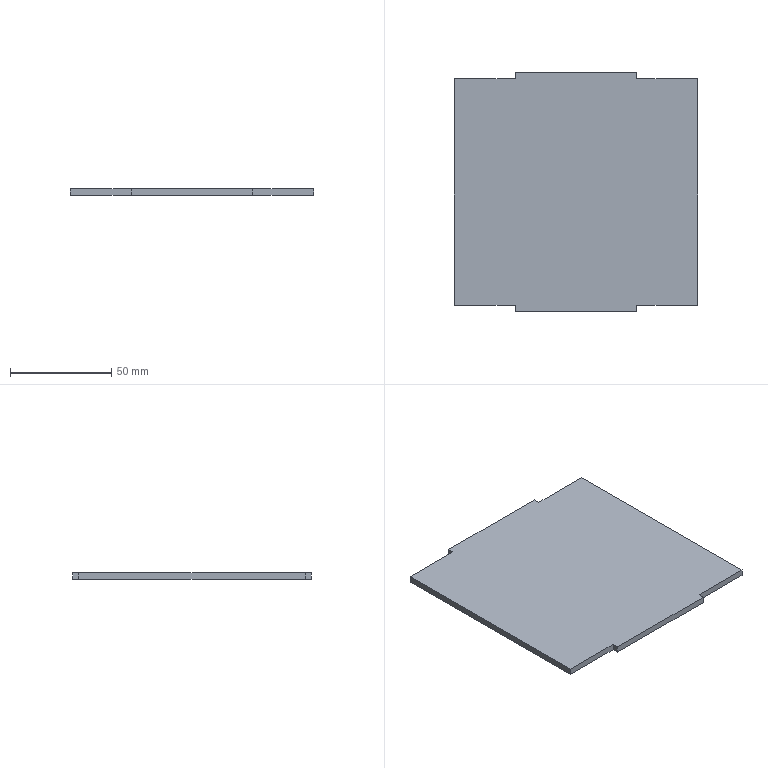Part | SolidWorks | features FlatPattern 1, SMBaseFlange 1, SheetMetal 1 | 1 solid | 14 faces | box 120 x 117.8 x 3.2 mm | volume 44083 mm3 | plane 14
STEP:
#1=CARTESIAN_POINT('',(120.,-19.503,0.));
#2=VERTEX_POINT('',#1);
#3=CARTESIAN_POINT('',(120.,92.297,0.));
#4=VERTEX_POINT('',#3);
#5=CARTESIAN_POINT('',(120.,92.297,0.));
#6=DIRECTION('',(0.,1.,0.));
#7=VECTOR('',#6,1000.);
#8=LINE('',#5,#7);
#9=EDGE_CURVE('',#2,#4,#8,.T.);
#10=ORIENTED_EDGE('',*,*,#9,.F.);
#11=CARTESIAN_POINT('',(120.,-19.503,-3.2));
#12=VERTEX_POINT('',#11);
#13=CARTESIAN_POINT('',(120.,-19.503,-3.2));
#14=DIRECTION('',(0.,0.,1.));
#15=VECTOR('',#14,1000.);
#16=LINE('',#13,#15);
#17=EDGE_CURVE('',#12,#2,#16,.T.);
#18=ORIENTED_EDGE('',*,*,#17,.F.);
#19=CARTESIAN_POINT('',(120.,92.297,-3.2));
#20=VERTEX_POINT('',#19);
#21=CARTESIAN_POINT('',(120.,92.297,-3.2));
#22=DIRECTION('',(0.,1.,0.));
#23=VECTOR('',#22,1000.);
#24=LINE('',#21,#23);
#25=EDGE_CURVE('',#12,#20,#24,.T.);
#26=ORIENTED_EDGE('',*,*,#25,.T.);
#27=CARTESIAN_POINT('',(120.,92.297,-3.2));
#28=DIRECTION('',(0.,0.,1.));
#29=VECTOR('',#28,1000.);
#30=LINE('',#27,#29);
#31=EDGE_CURVE('',#20,#4,#30,.T.);
#32=ORIENTED_EDGE('',*,*,#31,.T.);
#33=EDGE_LOOP('',(#10,#18,#26,#32));
#34=FACE_OUTER_BOUND('',#33,.T.);
#35=CARTESIAN_POINT('',(120.,92.297,-3.2));
#36=DIRECTION('',(1.,0.,0.));
#37=DIRECTION('',(0.,1.,0.));
#38=AXIS2_PLACEMENT_3D('',#35,#36,#37);
#39=PLANE('',#38);
#40=ADVANCED_FACE('',(#34),#39,.T.);
#41=CARTESIAN_POINT('',(90.,-19.503,0.));
#42=VERTEX_POINT('',#41);
#43=CARTESIAN_POINT('',(120.,-19.503,0.));
#44=DIRECTION('',(1.,0.,0.));
#45=VECTOR('',#44,1000.);
#46=LINE('',#43,#45);
#47=EDGE_CURVE('',#42,#2,#46,.T.);
#48=ORIENTED_EDGE('',*,*,#47,.F.);
#49=CARTESIAN_POINT('',(90.,-19.503,-3.2));
#50=VERTEX_POINT('',#49);
#51=CARTESIAN_POINT('',(90.,-19.503,-3.2));
#52=DIRECTION('',(0.,0.,1.));
#53=VECTOR('',#52,1000.);
#54=LINE('',#51,#53);
#55=EDGE_CURVE('',#50,#42,#54,.T.);
#56=ORIENTED_EDGE('',*,*,#55,.F.);
#57=CARTESIAN_POINT('',(120.,-19.503,-3.2));
#58=DIRECTION('',(1.,0.,0.));
#59=VECTOR('',#58,1000.);
#60=LINE('',#57,#59);
#61=EDGE_CURVE('',#50,#12,#60,.T.);
#62=ORIENTED_EDGE('',*,*,#61,.T.);
#63=ORIENTED_EDGE('',*,*,#17,.T.);
#64=EDGE_LOOP('',(#48,#56,#62,#63));
#65=FACE_OUTER_BOUND('',#64,.T.);
#66=CARTESIAN_POINT('',(120.,-19.503,-3.2));
#67=DIRECTION('',(0.,-1.,0.));
#68=DIRECTION('',(1.,0.,0.));
#69=AXIS2_PLACEMENT_3D('',#66,#67,#68);
#70=PLANE('',#69);
#71=ADVANCED_FACE('',(#65),#70,.T.);
#72=CARTESIAN_POINT('',(90.,-22.503,0.));
#73=VERTEX_POINT('',#72);
#74=CARTESIAN_POINT('',(90.,-19.503,0.));
#75=DIRECTION('',(0.,1.,0.));
#76=VECTOR('',#75,1000.);
#77=LINE('',#74,#76);
#78=EDGE_CURVE('',#73,#42,#77,.T.);
#79=ORIENTED_EDGE('',*,*,#78,.F.);
#80=CARTESIAN_POINT('',(90.,-22.503,-3.2));
#81=VERTEX_POINT('',#80);
#82=CARTESIAN_POINT('',(90.,-22.503,-3.2));
#83=DIRECTION('',(0.,0.,1.));
#84=VECTOR('',#83,1000.);
#85=LINE('',#82,#84);
#86=EDGE_CURVE('',#81,#73,#85,.T.);
#87=ORIENTED_EDGE('',*,*,#86,.F.);
#88=CARTESIAN_POINT('',(90.,-19.503,-3.2));
#89=DIRECTION('',(0.,1.,0.));
#90=VECTOR('',#89,1000.);
#91=LINE('',#88,#90);
#92=EDGE_CURVE('',#81,#50,#91,.T.);
#93=ORIENTED_EDGE('',*,*,#92,.T.);
#94=ORIENTED_EDGE('',*,*,#55,.T.);
#95=EDGE_LOOP('',(#79,#87,#93,#94));
#96=FACE_OUTER_BOUND('',#95,.T.);
#97=CARTESIAN_POINT('',(90.,-19.503,-3.2));
#98=DIRECTION('',(1.,0.,0.));
#99=DIRECTION('',(0.,0.,-1.));
#100=AXIS2_PLACEMENT_3D('',#97,#98,#99);
#101=PLANE('',#100);
#102=ADVANCED_FACE('',(#96),#101,.T.);
#103=CARTESIAN_POINT('',(30.,-22.503,0.));
#104=VERTEX_POINT('',#103);
#105=CARTESIAN_POINT('',(90.,-22.503,0.));
#106=DIRECTION('',(1.,0.,0.));
#107=VECTOR('',#106,1000.);
#108=LINE('',#105,#107);
#109=EDGE_CURVE('',#104,#73,#108,.T.);
#110=ORIENTED_EDGE('',*,*,#109,.F.);
#111=CARTESIAN_POINT('',(30.,-22.503,-3.2));
#112=VERTEX_POINT('',#111);
#113=CARTESIAN_POINT('',(30.,-22.503,-3.2));
#114=DIRECTION('',(0.,0.,1.));
#115=VECTOR('',#114,1000.);
#116=LINE('',#113,#115);
#117=EDGE_CURVE('',#112,#104,#116,.T.);
#118=ORIENTED_EDGE('',*,*,#117,.F.);
#119=CARTESIAN_POINT('',(90.,-22.503,-3.2));
#120=DIRECTION('',(1.,0.,0.));
#121=VECTOR('',#120,1000.);
#122=LINE('',#119,#121);
#123=EDGE_CURVE('',#112,#81,#122,.T.);
#124=ORIENTED_EDGE('',*,*,#123,.T.);
#125=ORIENTED_EDGE('',*,*,#86,.T.);
#126=EDGE_LOOP('',(#110,#118,#124,#125));
#127=FACE_OUTER_BOUND('',#126,.T.);
#128=CARTESIAN_POINT('',(90.,-22.503,-3.2));
#129=DIRECTION('',(0.,-1.,0.));
#130=DIRECTION('',(1.,0.,0.));
#131=AXIS2_PLACEMENT_3D('',#128,#129,#130);
#132=PLANE('',#131);
#133=ADVANCED_FACE('',(#127),#132,.T.);
#134=CARTESIAN_POINT('',(30.,-19.503,0.));
#135=VERTEX_POINT('',#134);
#136=CARTESIAN_POINT('',(30.,-22.503,0.));
#137=DIRECTION('',(0.,-1.,0.));
#138=VECTOR('',#137,1000.);
#139=LINE('',#136,#138);
#140=EDGE_CURVE('',#135,#104,#139,.T.);
#141=ORIENTED_EDGE('',*,*,#140,.F.);
#142=CARTESIAN_POINT('',(30.,-19.503,-3.2));
#143=VERTEX_POINT('',#142);
#144=CARTESIAN_POINT('',(30.,-19.503,-3.2));
#145=DIRECTION('',(0.,0.,1.));
#146=VECTOR('',#145,1000.);
#147=LINE('',#144,#146);
#148=EDGE_CURVE('',#143,#135,#147,.T.);
#149=ORIENTED_EDGE('',*,*,#148,.F.);
#150=CARTESIAN_POINT('',(30.,-22.503,-3.2));
#151=DIRECTION('',(0.,-1.,0.));
#152=VECTOR('',#151,1000.);
#153=LINE('',#150,#152);
#154=EDGE_CURVE('',#143,#112,#153,.T.);
#155=ORIENTED_EDGE('',*,*,#154,.T.);
#156=ORIENTED_EDGE('',*,*,#117,.T.);
#157=EDGE_LOOP('',(#141,#149,#155,#156));
#158=FACE_OUTER_BOUND('',#157,.T.);
#159=CARTESIAN_POINT('',(30.,-22.503,-3.2));
#160=DIRECTION('',(-1.,0.,0.));
#161=DIRECTION('',(0.,0.,1.));
#162=AXIS2_PLACEMENT_3D('',#159,#160,#161);
#163=PLANE('',#162);
#164=ADVANCED_FACE('',(#158),#163,.T.);
#165=CARTESIAN_POINT('',(0.,-19.503,0.));
#166=VERTEX_POINT('',#165);
#167=CARTESIAN_POINT('',(30.,-19.503,0.));
#168=DIRECTION('',(1.,0.,0.));
#169=VECTOR('',#168,1000.);
#170=LINE('',#167,#169);
#171=EDGE_CURVE('',#166,#135,#170,.T.);
#172=ORIENTED_EDGE('',*,*,#171,.F.);
#173=CARTESIAN_POINT('',(0.,-19.503,-3.2));
#174=VERTEX_POINT('',#173);
#175=CARTESIAN_POINT('',(0.,-19.503,-3.2));
#176=DIRECTION('',(0.,0.,1.));
#177=VECTOR('',#176,1000.);
#178=LINE('',#175,#177);
#179=EDGE_CURVE('',#174,#166,#178,.T.);
#180=ORIENTED_EDGE('',*,*,#179,.F.);
#181=CARTESIAN_POINT('',(30.,-19.503,-3.2));
#182=DIRECTION('',(1.,0.,0.));
#183=VECTOR('',#182,1000.);
#184=LINE('',#181,#183);
#185=EDGE_CURVE('',#174,#143,#184,.T.);
#186=ORIENTED_EDGE('',*,*,#185,.T.);
#187=ORIENTED_EDGE('',*,*,#148,.T.);
#188=EDGE_LOOP('',(#172,#180,#186,#187));
#189=FACE_OUTER_BOUND('',#188,.T.);
#190=CARTESIAN_POINT('',(30.,-19.503,-3.2));
#191=DIRECTION('',(0.,-1.,0.));
#192=DIRECTION('',(1.,0.,0.));
#193=AXIS2_PLACEMENT_3D('',#190,#191,#192);
#194=PLANE('',#193);
#195=ADVANCED_FACE('',(#189),#194,.T.);
#196=CARTESIAN_POINT('',(0.,92.297,0.));
#197=VERTEX_POINT('',#196);
#198=CARTESIAN_POINT('',(0.,92.297,0.));
#199=DIRECTION('',(0.,-1.,0.));
#200=VECTOR('',#199,1000.);
#201=LINE('',#198,#200);
#202=EDGE_CURVE('',#197,#166,#201,.T.);
#203=ORIENTED_EDGE('',*,*,#202,.F.);
#204=CARTESIAN_POINT('',(0.,92.297,-3.2));
#205=VERTEX_POINT('',#204);
#206=CARTESIAN_POINT('',(0.,92.297,-3.2));
#207=DIRECTION('',(0.,0.,1.));
#208=VECTOR('',#207,1000.);
#209=LINE('',#206,#208);
#210=EDGE_CURVE('',#205,#197,#209,.T.);
#211=ORIENTED_EDGE('',*,*,#210,.F.);
#212=CARTESIAN_POINT('',(0.,92.297,-3.2));
#213=DIRECTION('',(0.,-1.,0.));
#214=VECTOR('',#213,1000.);
#215=LINE('',#212,#214);
#216=EDGE_CURVE('',#205,#174,#215,.T.);
#217=ORIENTED_EDGE('',*,*,#216,.T.);
#218=ORIENTED_EDGE('',*,*,#179,.T.);
#219=EDGE_LOOP('',(#203,#211,#217,#218));
#220=FACE_OUTER_BOUND('',#219,.T.);
#221=CARTESIAN_POINT('',(0.,92.297,-3.2));
#222=DIRECTION('',(-1.,0.,0.));
#223=DIRECTION('',(0.,0.,1.));
#224=AXIS2_PLACEMENT_3D('',#221,#222,#223);
#225=PLANE('',#224);
#226=ADVANCED_FACE('',(#220),#225,.T.);
#227=CARTESIAN_POINT('',(30.,92.297,0.));
#228=VERTEX_POINT('',#227);
#229=CARTESIAN_POINT('',(30.,92.297,0.));
#230=DIRECTION('',(-1.,0.,0.));
#231=VECTOR('',#230,1000.);
#232=LINE('',#229,#231);
#233=EDGE_CURVE('',#228,#197,#232,.T.);
#234=ORIENTED_EDGE('',*,*,#233,.F.);
#235=CARTESIAN_POINT('',(30.,92.297,-3.2));
#236=VERTEX_POINT('',#235);
#237=CARTESIAN_POINT('',(30.,92.297,-3.2));
#238=DIRECTION('',(0.,0.,1.));
#239=VECTOR('',#238,1000.);
#240=LINE('',#237,#239);
#241=EDGE_CURVE('',#236,#228,#240,.T.);
#242=ORIENTED_EDGE('',*,*,#241,.F.);
#243=CARTESIAN_POINT('',(30.,92.297,-3.2));
#244=DIRECTION('',(-1.,0.,0.));
#245=VECTOR('',#244,1000.);
#246=LINE('',#243,#245);
#247=EDGE_CURVE('',#236,#205,#246,.T.);
#248=ORIENTED_EDGE('',*,*,#247,.T.);
#249=ORIENTED_EDGE('',*,*,#210,.T.);
#250=EDGE_LOOP('',(#234,#242,#248,#249));
#251=FACE_OUTER_BOUND('',#250,.T.);
#252=CARTESIAN_POINT('',(30.,92.297,-3.2));
#253=DIRECTION('',(0.,1.,0.));
#254=DIRECTION('',(-1.,0.,0.));
#255=AXIS2_PLACEMENT_3D('',#252,#253,#254);
#256=PLANE('',#255);
#257=ADVANCED_FACE('',(#251),#256,.T.);
#258=CARTESIAN_POINT('',(30.,95.297,0.));
#259=VERTEX_POINT('',#258);
#260=CARTESIAN_POINT('',(30.,95.297,0.));
#261=DIRECTION('',(0.,-1.,0.));
#262=VECTOR('',#261,1000.);
#263=LINE('',#260,#262);
#264=EDGE_CURVE('',#259,#228,#263,.T.);
#265=ORIENTED_EDGE('',*,*,#264,.F.);
#266=CARTESIAN_POINT('',(30.,95.297,-3.2));
#267=VERTEX_POINT('',#266);
#268=CARTESIAN_POINT('',(30.,95.297,-3.2));
#269=DIRECTION('',(0.,0.,1.));
#270=VECTOR('',#269,1000.);
#271=LINE('',#268,#270);
#272=EDGE_CURVE('',#267,#259,#271,.T.);
#273=ORIENTED_EDGE('',*,*,#272,.F.);
#274=CARTESIAN_POINT('',(30.,95.297,-3.2));
#275=DIRECTION('',(0.,-1.,0.));
#276=VECTOR('',#275,1000.);
#277=LINE('',#274,#276);
#278=EDGE_CURVE('',#267,#236,#277,.T.);
#279=ORIENTED_EDGE('',*,*,#278,.T.);
#280=ORIENTED_EDGE('',*,*,#241,.T.);
#281=EDGE_LOOP('',(#265,#273,#279,#280));
#282=FACE_OUTER_BOUND('',#281,.T.);
#283=CARTESIAN_POINT('',(30.,95.297,-3.2));
#284=DIRECTION('',(-1.,0.,0.));
#285=DIRECTION('',(0.,0.,1.));
#286=AXIS2_PLACEMENT_3D('',#283,#284,#285);
#287=PLANE('',#286);
#288=ADVANCED_FACE('',(#282),#287,.T.);
#289=CARTESIAN_POINT('',(90.,95.297,0.));
#290=VERTEX_POINT('',#289);
#291=CARTESIAN_POINT('',(90.,95.297,0.));
#292=DIRECTION('',(-1.,0.,0.));
#293=VECTOR('',#292,1000.);
#294=LINE('',#291,#293);
#295=EDGE_CURVE('',#290,#259,#294,.T.);
#296=ORIENTED_EDGE('',*,*,#295,.F.);
#297=CARTESIAN_POINT('',(90.,95.297,-3.2));
#298=VERTEX_POINT('',#297);
#299=CARTESIAN_POINT('',(90.,95.297,-3.2));
#300=DIRECTION('',(0.,0.,1.));
#301=VECTOR('',#300,1000.);
#302=LINE('',#299,#301);
#303=EDGE_CURVE('',#298,#290,#302,.T.);
#304=ORIENTED_EDGE('',*,*,#303,.F.);
#305=CARTESIAN_POINT('',(90.,95.297,-3.2));
#306=DIRECTION('',(-1.,0.,0.));
#307=VECTOR('',#306,1000.);
#308=LINE('',#305,#307);
#309=EDGE_CURVE('',#298,#267,#308,.T.);
#310=ORIENTED_EDGE('',*,*,#309,.T.);
#311=ORIENTED_EDGE('',*,*,#272,.T.);
#312=EDGE_LOOP('',(#296,#304,#310,#311));
#313=FACE_OUTER_BOUND('',#312,.T.);
#314=CARTESIAN_POINT('',(90.,95.297,-3.2));
#315=DIRECTION('',(0.,1.,0.));
#316=DIRECTION('',(-1.,0.,0.));
#317=AXIS2_PLACEMENT_3D('',#314,#315,#316);
#318=PLANE('',#317);
#319=ADVANCED_FACE('',(#313),#318,.T.);
#320=CARTESIAN_POINT('',(90.,92.297,0.));
#321=VERTEX_POINT('',#320);
#322=CARTESIAN_POINT('',(90.,92.297,0.));
#323=DIRECTION('',(0.,1.,0.));
#324=VECTOR('',#323,1000.);
#325=LINE('',#322,#324);
#326=EDGE_CURVE('',#321,#290,#325,.T.);
#327=ORIENTED_EDGE('',*,*,#326,.F.);
#328=CARTESIAN_POINT('',(90.,92.297,-3.2));
#329=VERTEX_POINT('',#328);
#330=CARTESIAN_POINT('',(90.,92.297,-3.2));
#331=DIRECTION('',(0.,0.,1.));
#332=VECTOR('',#331,1000.);
#333=LINE('',#330,#332);
#334=EDGE_CURVE('',#329,#321,#333,.T.);
#335=ORIENTED_EDGE('',*,*,#334,.F.);
#336=CARTESIAN_POINT('',(90.,92.297,-3.2));
#337=DIRECTION('',(0.,1.,0.));
#338=VECTOR('',#337,1000.);
#339=LINE('',#336,#338);
#340=EDGE_CURVE('',#329,#298,#339,.T.);
#341=ORIENTED_EDGE('',*,*,#340,.T.);
#342=ORIENTED_EDGE('',*,*,#303,.T.);
#343=EDGE_LOOP('',(#327,#335,#341,#342));
#344=FACE_OUTER_BOUND('',#343,.T.);
#345=CARTESIAN_POINT('',(90.,92.297,-3.2));
#346=DIRECTION('',(1.,0.,0.));
#347=DIRECTION('',(0.,0.,-1.));
#348=AXIS2_PLACEMENT_3D('',#345,#346,#347);
#349=PLANE('',#348);
#350=ADVANCED_FACE('',(#344),#349,.T.);
#351=CARTESIAN_POINT('',(120.,92.297,0.));
#352=DIRECTION('',(-1.,0.,0.));
#353=VECTOR('',#352,1000.);
#354=LINE('',#351,#353);
#355=EDGE_CURVE('',#4,#321,#354,.T.);
#356=ORIENTED_EDGE('',*,*,#355,.F.);
#357=ORIENTED_EDGE('',*,*,#31,.F.);
#358=CARTESIAN_POINT('',(120.,92.297,-3.2));
#359=DIRECTION('',(-1.,0.,0.));
#360=VECTOR('',#359,1000.);
#361=LINE('',#358,#360);
#362=EDGE_CURVE('',#20,#329,#361,.T.);
#363=ORIENTED_EDGE('',*,*,#362,.T.);
#364=ORIENTED_EDGE('',*,*,#334,.T.);
#365=EDGE_LOOP('',(#356,#357,#363,#364));
#366=FACE_OUTER_BOUND('',#365,.T.);
#367=CARTESIAN_POINT('',(120.,92.297,-3.2));
#368=DIRECTION('',(0.,1.,0.));
#369=DIRECTION('',(0.,0.,1.));
#370=AXIS2_PLACEMENT_3D('',#367,#368,#369);
#371=PLANE('',#370);
#372=ADVANCED_FACE('',(#366),#371,.T.);
#373=ORIENTED_EDGE('',*,*,#25,.F.);
#374=ORIENTED_EDGE('',*,*,#61,.F.);
#375=ORIENTED_EDGE('',*,*,#92,.F.);
#376=ORIENTED_EDGE('',*,*,#123,.F.);
#377=ORIENTED_EDGE('',*,*,#154,.F.);
#378=ORIENTED_EDGE('',*,*,#185,.F.);
#379=ORIENTED_EDGE('',*,*,#216,.F.);
#380=ORIENTED_EDGE('',*,*,#247,.F.);
#381=ORIENTED_EDGE('',*,*,#278,.F.);
#382=ORIENTED_EDGE('',*,*,#309,.F.);
#383=ORIENTED_EDGE('',*,*,#340,.F.);
#384=ORIENTED_EDGE('',*,*,#362,.F.);
#385=EDGE_LOOP('',(#373,#374,#375,#376,#377,#378,#379,#380,#381,#382,#383,#384));
#386=FACE_OUTER_BOUND('',#385,.T.);
#387=CARTESIAN_POINT('',(0.,0.,-3.2));
#388=DIRECTION('',(0.,0.,-1.));
#389=DIRECTION('',(-1.,0.,0.));
#390=AXIS2_PLACEMENT_3D('',#387,#388,#389);
#391=PLANE('',#390);
#392=ADVANCED_FACE('',(#386),#391,.T.);
#393=ORIENTED_EDGE('',*,*,#9,.T.);
#394=ORIENTED_EDGE('',*,*,#355,.T.);
#395=ORIENTED_EDGE('',*,*,#326,.T.);
#396=ORIENTED_EDGE('',*,*,#295,.T.);
#397=ORIENTED_EDGE('',*,*,#264,.T.);
#398=ORIENTED_EDGE('',*,*,#233,.T.);
#399=ORIENTED_EDGE('',*,*,#202,.T.);
#400=ORIENTED_EDGE('',*,*,#171,.T.);
#401=ORIENTED_EDGE('',*,*,#140,.T.);
#402=ORIENTED_EDGE('',*,*,#109,.T.);
#403=ORIENTED_EDGE('',*,*,#78,.T.);
#404=ORIENTED_EDGE('',*,*,#47,.T.);
#405=EDGE_LOOP('',(#393,#394,#395,#396,#397,#398,#399,#400,#401,#402,#403,#404));
#406=FACE_OUTER_BOUND('',#405,.T.);
#407=CARTESIAN_POINT('',(0.,0.,0.));
#408=DIRECTION('',(0.,0.,-1.));
#409=DIRECTION('',(-1.,0.,0.));
#410=AXIS2_PLACEMENT_3D('',#407,#408,#409);
#411=PLANE('',#410);
#412=ADVANCED_FACE('',(#406),#411,.F.);
#413=CLOSED_SHELL('',(#40,#71,#102,#133,#164,#195,#226,#257,#288,#319,#350,#372,#392,#412));
#414=MANIFOLD_SOLID_BREP('',#413);
#415=CARTESIAN_POINT('',(0.,0.,0.));
#416=DIRECTION('',(0.,0.,1.));
#417=DIRECTION('',(1.,0.,0.));
#418=AXIS2_PLACEMENT_3D('',#415,#416,#417);
#419=(LENGTH_UNIT()NAMED_UNIT(*)SI_UNIT(.MILLI.,.METRE.));
#420=UNCERTAINTY_MEASURE_WITH_UNIT(LENGTH_MEASURE(0.00001),#419,'','');
#421=(NAMED_UNIT(*)PLANE_ANGLE_UNIT()SI_UNIT($,.RADIAN.));
#422=(NAMED_UNIT(*)SI_UNIT($,.STERADIAN.)SOLID_ANGLE_UNIT());
#423=(GEOMETRIC_REPRESENTATION_CONTEXT(3)GLOBAL_UNCERTAINTY_ASSIGNED_CONTEXT((#420))GLOBAL_UNIT_ASSIGNED_CONTEXT((#419,#421,#422))REPRESENTATION_CONTEXT('',''));
#424=ADVANCED_BREP_SHAPE_REPRESENTATION('',(#414,#418),#423);